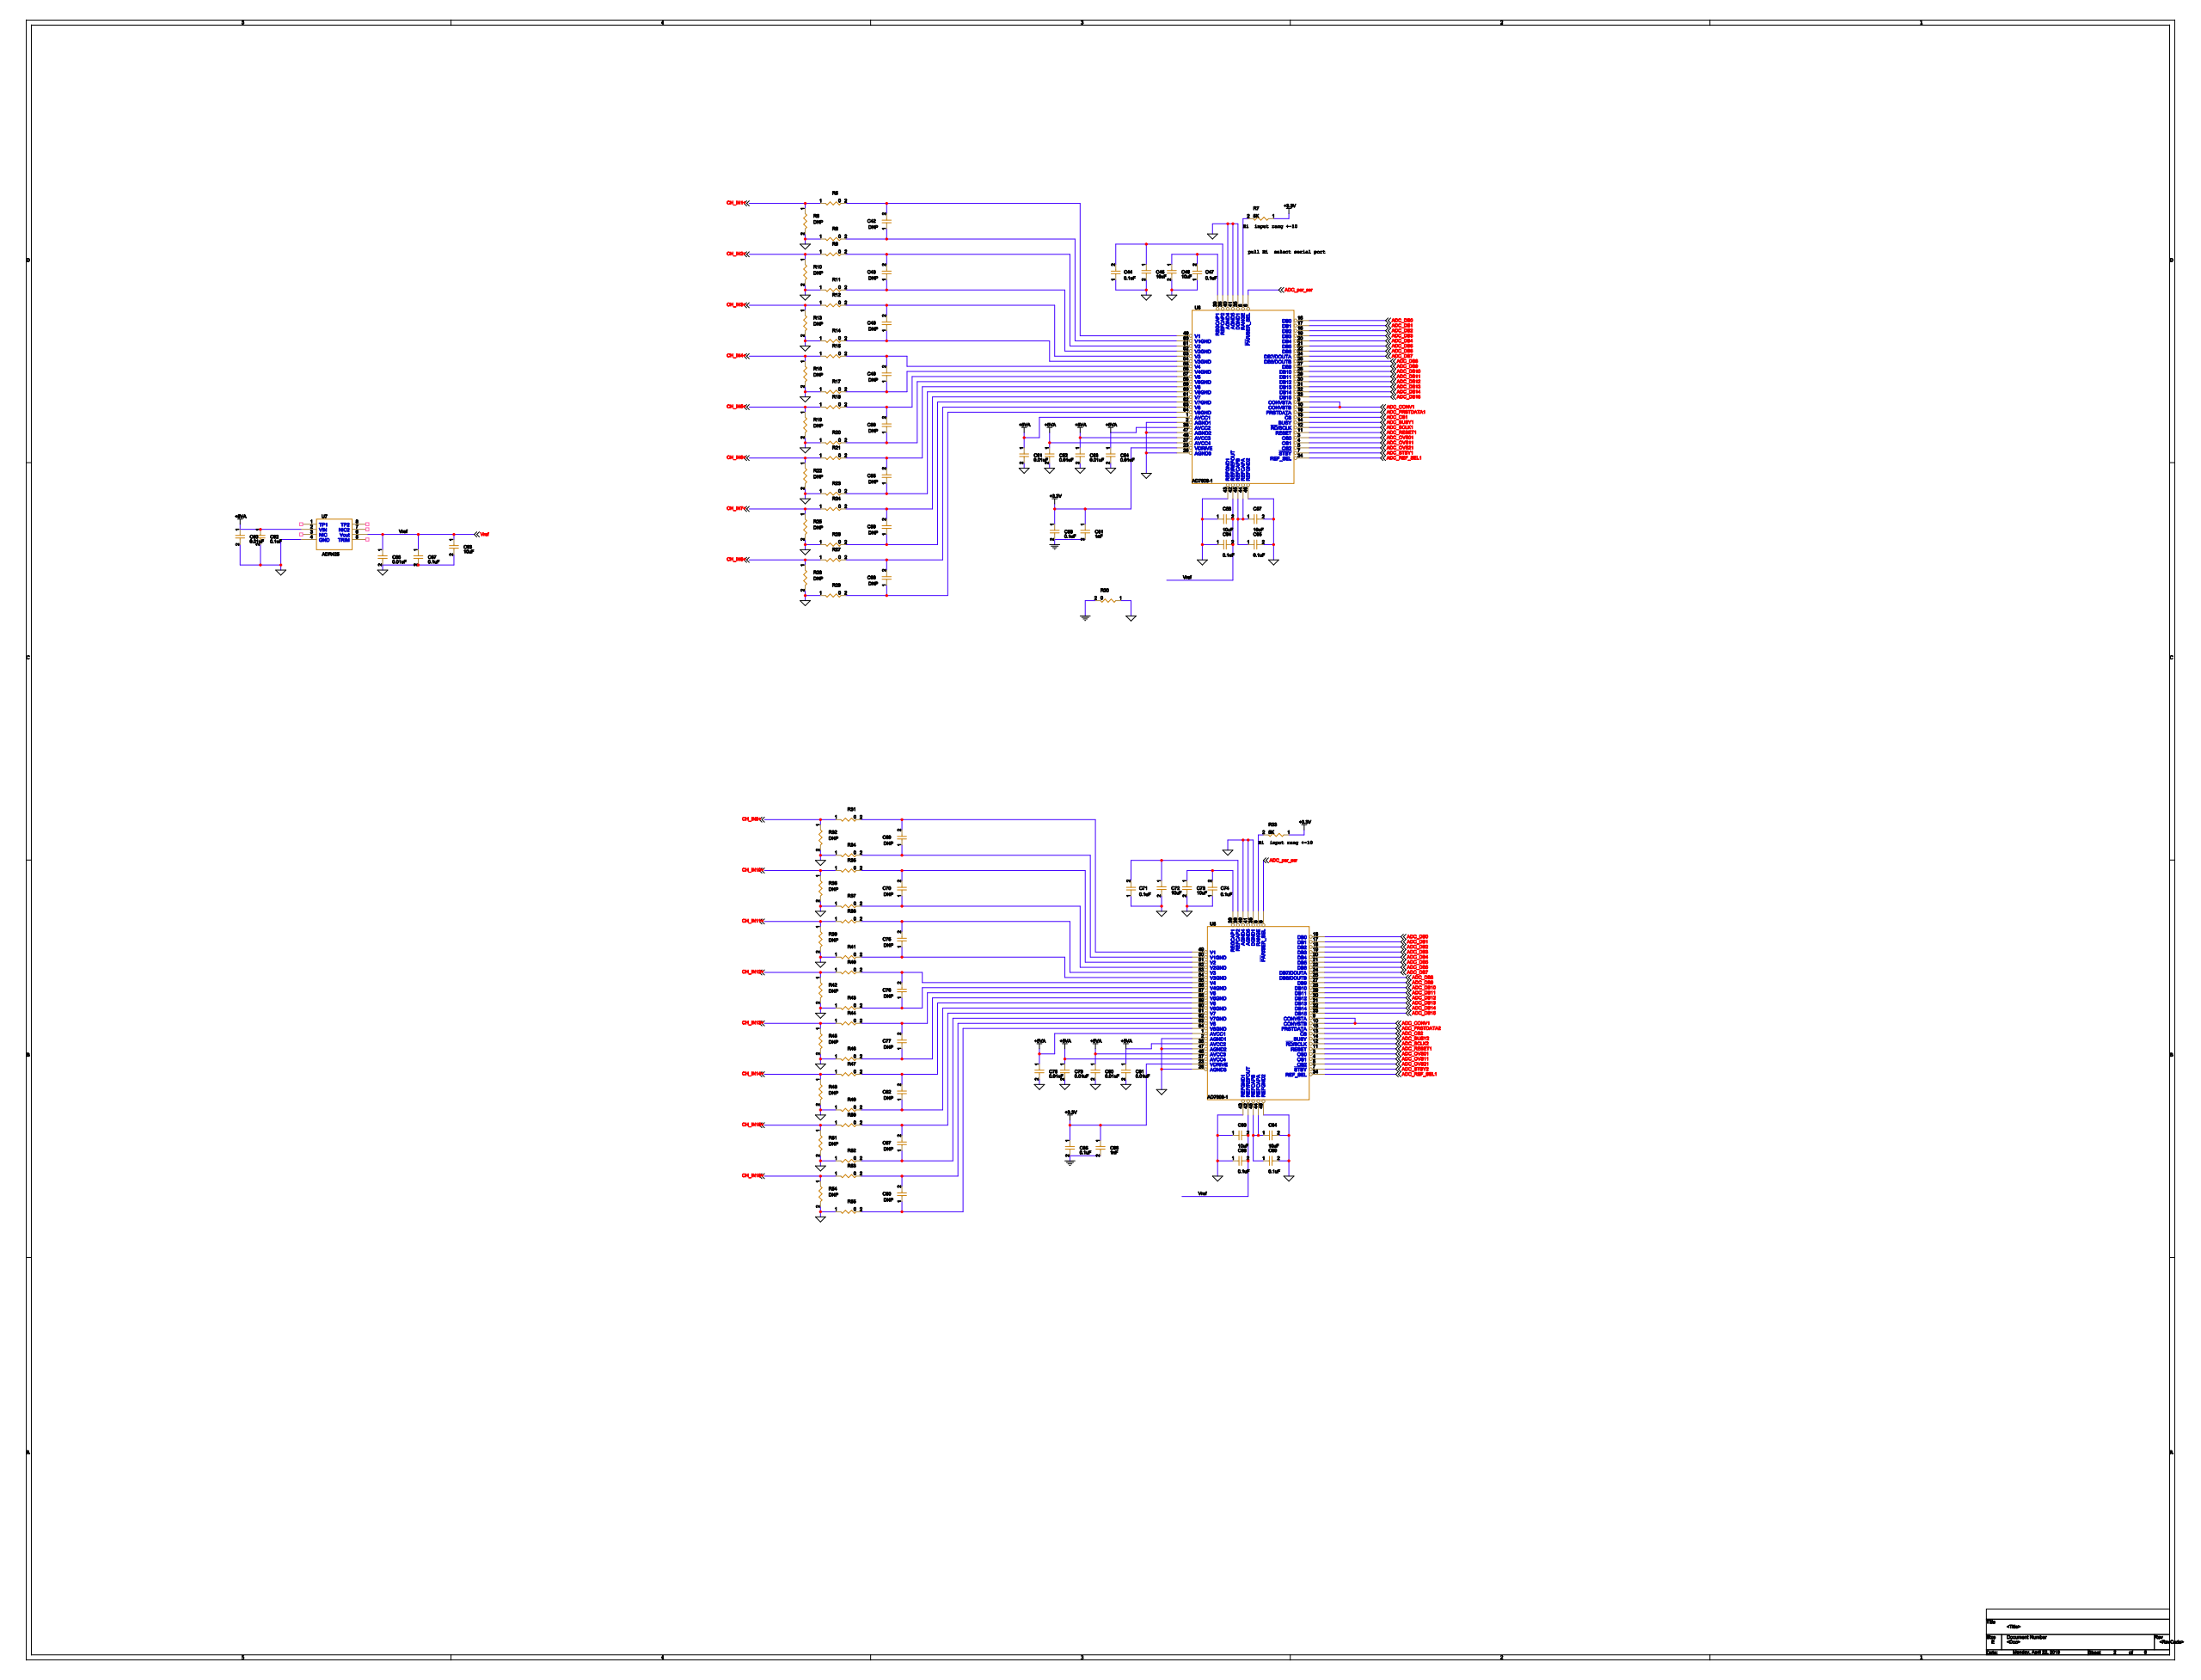Circuit board | Cadence Allegro | 362 parts | 391 nets | one sheet of the schematic
Parts on this sheet (reference | value | footprint):
C42 | DNP | 0805
C43 | DNP | 0805
C44 | 0.1uF | 1206
C45 | 10uF | 6032
C46 | 10uF | 6032
C47 | 0.1uF | 1206
C48 | DNP | 0805
C49 | DNP | 0805
C50 | DNP | 0805
C51 | 0.01uF | 0805
C52 | 0.01uF | 0805
C53 | 0.01uF | 0805
C54 | 0.01uF | 0805
C55 | DNP | 0805
C56 | 10uF | 6032
C57 | 10uF | 6032
C58 | 0.1uF | 1206
C59 | DNP | 0805
C60 | 0.01uF | 0805
C61 | 1nF | 0805
C62 | 0.1uF | 1206
C63 | 10uF | 6032
C64 | 0.1uF | 1206
C65 | 0.1uF | 1206
C66 | 0.01uF | 0805
C67 | 0.1uF | 1206
C68 | DNP | 0805
C69 | DNP | 0805
C70 | DNP | 0805
C71 | 0.1uF | 1206
C72 | 10uF | 6032
C73 | 10uF | 6032
C74 | 0.1uF | 1206
C75 | DNP | 0805
C76 | DNP | 0805
C77 | DNP | 0805
C78 | 0.01uF | 0805
C79 | 0.01uF | 0805
C80 | 0.01uF | 0805
C81 | 0.01uF | 0805
C82 | DNP | 0805
C83 | 10uF | 6032
C84 | 10uF | 6032
C85 | 0.1uF | 1206
C86 | 1nF | 0805
C87 | DNP | 0805
C88 | 0.1uF | 1206
C89 | 0.1uF | 1206
C90 | DNP | 0805
R5 | 0 | 0805
R6 | DNP | 0805
R7 | 5K | 0805
R8 | 0 | 0805
R9 | 0 | 0805
R10 | DNP | 0805
R11 | 0 | 0805
R12 | 0 | 0805
R13 | DNP | 0805
R14 | 0 | 0805
R15 | 0 | 0805
R16 | DNP | 0805
R17 | 0 | 0805
R18 | 0 | 0805
R19 | DNP | 0805
R20 | 0 | 0805
R21 | 0 | 0805
R22 | DNP | 0805
R23 | 0 | 0805
R24 | 0 | 0805
R25 | DNP | 0805
R26 | 0 | 0805
R27 | 0 | 0805
R28 | DNP | 0805
R29 | 0 | 0805
R30 | 0 | 0805
R31 | 0 | 0805
R32 | DNP | 0805
R33 | 5K | 0805
R34 | 0 | 0805
R35 | 0 | 0805
R36 | DNP | 0805
R37 | 0 | 0805
R38 | 0 | 0805
R39 | DNP | 0805
R40 | 0 | 0805
R41 | 0 | 0805
R42 | DNP | 0805
R43 | 0 | 0805
R44 | 0 | 0805
R45 | DNP | 0805
R46 | 0 | 0805
R47 | 0 | 0805
R48 | DNP | 0805
R49 | 0 | 0805
R50 | 0 | 0805
R51 | DNP | 0805
R52 | 0 | 0805
R53 | 0 | 0805
R54 | DNP | 0805
R55 | 0 | 0805
U6 | AD7608-1 | TQFP64
U7 | ADR425 | SO-8
U8 | AD7608-1 | TQFP64
Nets of these parts (net: part-pin ...):
VREF: C56-2 C63-1 C64-2 C66-1 C67-1 C83-2 C88-2 U7-6 U6-42 U8-42
+3.3V: C58-1 C61-1 C85-1 C86-1 R7-1 R33-1 U6-23 U8-23
DGND: C58-2 C61-2 C85-2 C86-2 R30-2
AGND: C44-1 C45-2 C46-2 C47-1 C51-2 C52-2 C53-2 C54-2 C56-1 C57-2 C60-2 C62-2 C63-2 C64-1 C65-2 C66-2 C67-2 C71-1 C72-2 C73-2 C74-1 C78-2 C79-2 C80-2 C81-2 C83-1 C84-2 C88-1 C89-2 R6-2 R8-1 R10-2 R11-1 R13-2 R14-1 R16-2 R17-1 R19-2 R20-1 R22-2 R23-1 R25-2 R26-1 R28-2 R29-1 R30-1 R32-2 R34-1 R36-2 R37-1 R39-2 R41-1 R42-2 R43-1 R45-2 R46-1 R48-2 R49-1 R51-2 R52-1 R54-2 R55-1 U7-4 U6-2 U6-26 U6-35 U6-40 U6-41 U6-43 U6-46 U6-47 U8-2 U8-26 U8-35 U8-40 U8-41 U8-43 U8-46 U8-47
+5VA: C51-1 C52-1 C53-1 C54-1 C60-1 C62-1 C78-1 C79-1 C80-1 C81-1 U7-2 U6-1 U6-37 U6-38 U6-48 U8-1 U8-37 U8-38 U8-48
ADC_BUSY2: U8-14
ADC_CONV1: U6-9 U6-10 U8-9 U8-10
ADC_DB0: U6-16 U8-16
ADC_DB1: U6-17 U8-17
ADC_DB10: U6-28 U8-28
ADC_DB11: U6-29 U8-29
ADC_DB12: U6-30 U8-30
ADC_DB13: U6-31 U8-31
ADC_DB14: U6-32 U8-32
ADC_DB15: U6-33 U8-33
ADC_DB2: U6-18 U8-18
ADC_DB3: U6-19 U8-19
ADC_DB4: U6-20 U8-20
ADC_DB5: U6-21 U8-21
ADC_DB6: U6-22 U8-22
ADC_DB7: U6-24 U8-24
ADC_DB8: U6-25 U8-25
ADC_DB9: U6-27 U8-27
ADC_FRSTDATA2: U8-15
ADC_OVS01: U6-3 U8-3
ADC_OVS11: U6-4 U8-4
ADC_OVS21: U6-5 U8-5
N17370295: R33-2 U8-8
N17370344: C71-2 C72-1 U8-36
N17371144: C84-1 C89-1 U8-44 U8-45
ADC_REF_SEL1: U6-34 U8-34
N17370387: C73-1 C74-2 U8-39
ADC_RESET1: U6-11 U8-11
ADC_STBY2: U8-7
N17370257: C69-2 R31-2 U8-49
N17370315: C69-1 R34-2 U8-50
N17370379: C70-2 R35-2 U8-51
N17370445: C70-1 R37-2 U8-52
N17370511: C75-2 R38-2 U8-53
N17370619: C75-1 R41-2 U8-54
N17370691: C76-2 R40-2 U8-55
N17370733: C76-1 R43-2 U8-56
N17370743: C77-2 R44-2 U8-57
N17370753: C77-1 R46-2 U8-58
N17370775: C82-2 R47-2 U8-59
N17370792: C82-1 R49-2 U8-60
N17370800: C87-2 R50-2 U8-61
N17370818: C87-1 R52-2 U8-62
N17370843: C90-2 R53-2 U8-63
N17370855: C90-1 R55-2 U8-64
ADC_CS2: U8-13
ADC_SCLK2: U8-12
ADC_BUSY1: U6-14
ADC_FRSTDATA1: U6-15
N17357145: R7-2 U6-8
N17355772: C44-2 C45-1 U6-36
N17358216: C57-1 C65-1 U6-44 U6-45
N17355763: C46-1 C47-2 U6-39
ADC_STBY1: U6-7
N17364330: C42-2 R5-2 U6-49
N17364351: C42-1 R8-2 U6-50
N17364667: C43-2 R9-2 U6-51
N17364687: C43-1 R11-2 U6-52
N17364801: C48-2 R12-2 U6-53
N17364821: C48-1 R14-2 U6-54
N17364943: C49-2 R15-2 U6-55
N17364963: C49-1 R17-2 U6-56
N17365249: C50-2 R18-2 U6-57
N17365269: C50-1 R20-2 U6-58
N17365303: C55-2 R21-2 U6-59
N17365323: C55-1 R23-2 U6-60
N17365357: C59-2 R24-2 U6-61
N17365377: C59-1 R26-2 U6-62
N17365411: C68-2 R27-2 U6-63
N17365431: C68-1 R29-2 U6-64
ADC_CS1: U6-13
ADC_SCLK1: U6-12
CH_IN13+: R44-1 R45-1
CH_IN14+: R47-1 R48-1
CH_IN15+: R50-1 R51-1
CH_IN16+: R53-1 R54-1
CH_IN9+: R31-1 R32-1
CH_IN10+: R35-1 R36-1
CH_IN11+: R38-1 R39-1
CH_IN12+: R40-1 R42-1
CH_IN5+: R18-1 R19-1
CH_IN6+: R21-1 R22-1
CH_IN7+: R24-1 R25-1
CH_IN8+: R27-1 R28-1
CH_IN1+: R5-1 R6-1
CH_IN2+: R9-1 R10-1
CH_IN3+: R12-1 R13-1
CH_IN4+: R15-1 R16-1